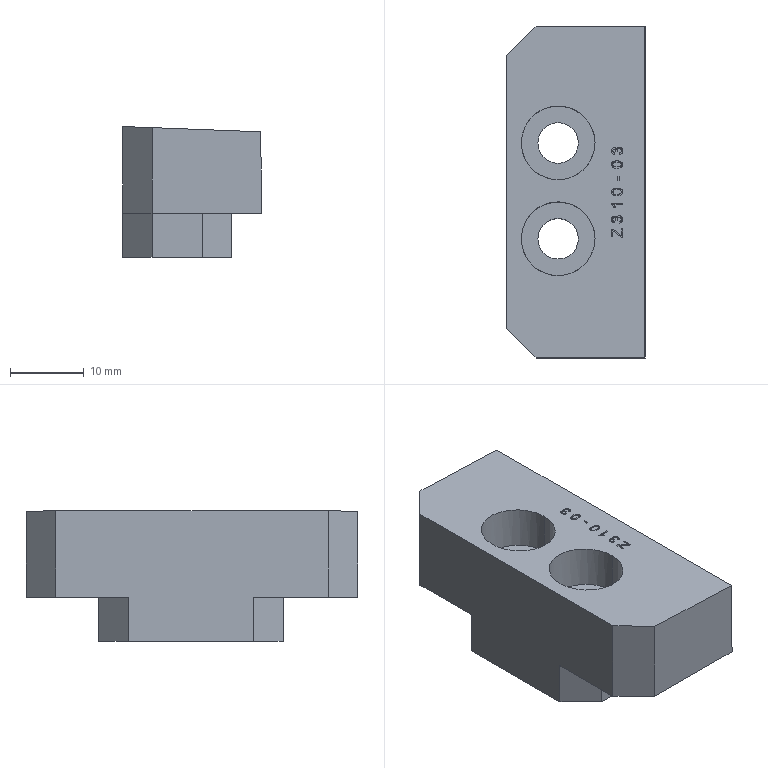Part | Creo | 1 solid | 160 faces | box 18.845 x 45 x 17.759 mm | volume 10002 mm3 | other 107 | plane 44 | cylinder 9 | commonest cylinder face diameters 5.5 x4 10 x4 20.538 x1